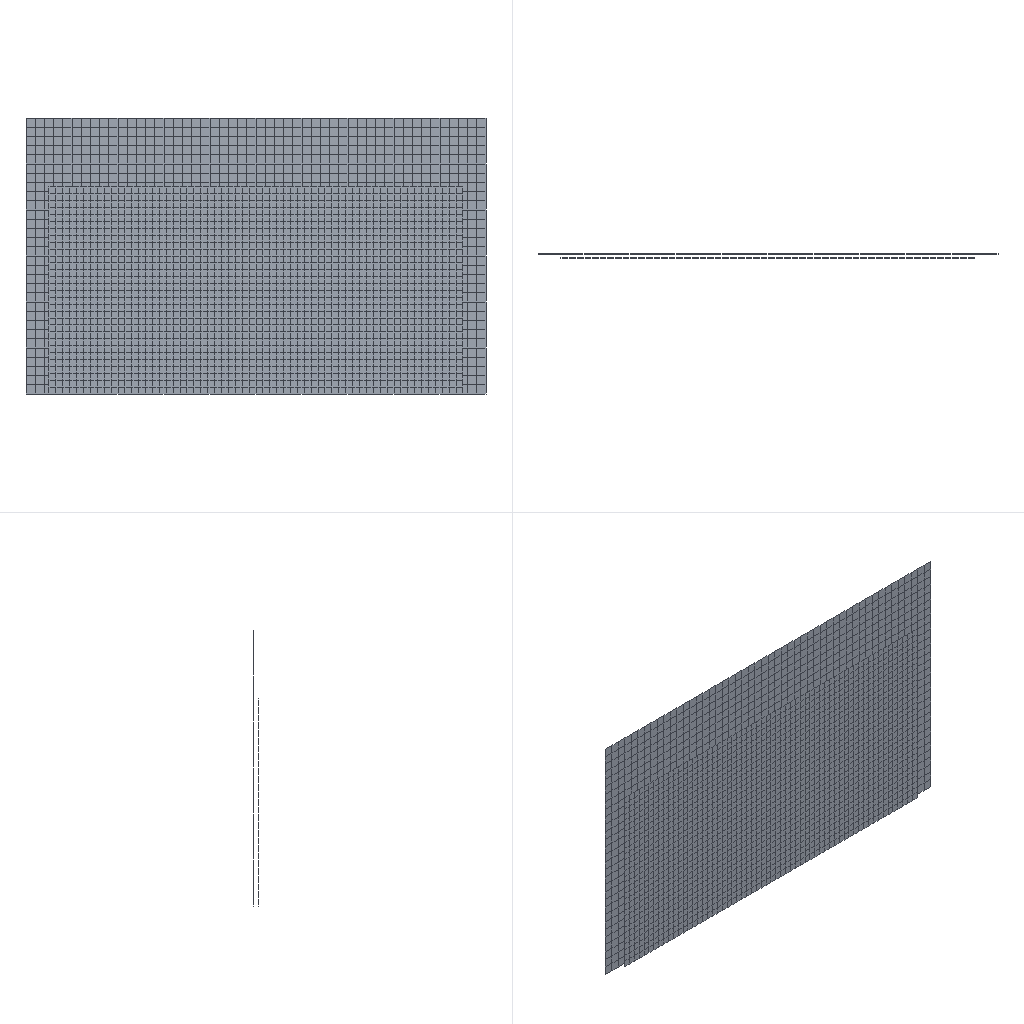Simulation study | abaqus
Set-up summary:
category,name,step,type,value,unit,region
solver,abaqus,,Abaqus/CAE 2024
units,mm-N-s-tonne (MPa),,inferred,E=70000 density=2.7e-09
analysis,forming step,,dynamic explicit,nlgeom=True; time_period=0.1
mesh,nodes,,,3941
mesh,elements,,,3720
element_type,S4R,,,3300
element_type,R3D4,,,420
material,banliao,,E,70000
material,banliao,,nu,0.33
material,banliao,,density,2.7e-09
material,banliao,,yield,131
material,banliao,,behaviors,plastic
material,xiangpi,,density,1.6e-09
material,xiangpi,,behaviors,hyperelastic
section,banliao,,shell section,2,,_PickedSet2
section,xiangpi,,shell section,10,,_PickedSet4
load,pressure,forming step,pressure,-5,,Surf-1
bc,fixdown,initial,encastre,[dofs=ENCASTRE],,down
contact,general,initial,general contact,interaction=Friction; friction=0.1; behavior=hard
constraint,rigid body,,,1
Abaqus input file, long lists of numbers shortened:
*Heading
** Job name: deck Model name: Model-1
** Generated by: Abaqus/CAE 2024
*Preprint, echo=NO, model=NO, history=NO, contact=NO
**
** PARTS
**
*Part, name=banliao
*Node
      1,         450.,         150.,         450.
      2,         435.,         150.,         450.
** (1889 more lines like these left out)
*Element, type=S4R
   1,    1,    2,   63,   62
   2,    2,    3,   64,   63
** (1798 more lines like these left out)
*Nset, nset=_PickedSet2, internal, generate
    1,  1891,     1
*Elset, elset=_PickedSet2, internal, generate
    1,  1800,     1
*Nset, nset=bl, generate
    1,  1891,     1
*Elset, elset=bl, generate
    1,  1800,     1
** Section: AIsection
*Shell Section, elset=_PickedSet2, material=banliao
2., 5
*End Part
**
*Part, name=muju
*Node
      1,        -240.,           0.,         500.
      2,        -250.,         -10.,         500.
** (466 more lines like these left out)
*Element, type=R3D4
 1,   1,  17, 161,  44
 2,  17,  18, 162, 161
** (418 more lines like these left out)
*Node
    469,         250.,        -150.,         250.
*Nset, nset=muju-RefPt_, internal
469,
*Nset, nset=down
 469,
*Elset, elset=muju, generate
   1,  420,    1
*End Part
**
*Part, name=xiangpi
*Node
      1,         500.,         250.,         600.
      2,         480.,         250.,         600.
** (1579 more lines like these left out)
*Element, type=S4R
   1,    1,    2,   53,   52
   2,    2,    3,   54,   53
** (1498 more lines like these left out)
*Nset, nset=xp, generate
    1,  1581,     1
*Elset, elset=xp, generate
    1,  1500,     1
*Nset, nset=_PickedSet3, internal, generate
    1,  1581,     1
*Elset, elset=_PickedSet3, internal, generate
    1,  1500,     1
*Nset, nset=_PickedSet4, internal, generate
    1,  1581,     1
*Elset, elset=_PickedSet4, internal, generate
    1,  1500,     1
** Section: Rub-section
*Shell Section, elset=_PickedSet4, material=xiangpi, controls=EC-1
10., 5
*End Part
**
**
** ASSEMBLY
**
*Assembly, name=Assembly
**
*Instance, name=banliao-1, part=banliao
          0.,        -148.,           0.
*End Instance
**
*Instance, name=muju-1, part=muju
*End Instance
**
*Instance, name=xiangpi-1, part=xiangpi
          0.,        -239.,           0.
*End Instance
**
*Nset, nset=down, instance=muju-1
 469,
*Elset, elset=_Surf-1_SPOS, internal, instance=xiangpi-1, generate
    1,  1500,     1
*Surface, type=ELEMENT, name=Surf-1
_Surf-1_SPOS, SPOS
*Rigid Body, ref node=muju-1.muju-RefPt_, elset=muju-1.muju
*End Assembly
**
** ELEMENT CONTROLS
**
*Section Controls, name=EC-1, hourglass=ENHANCED
1., 1., 1.
*Amplitude, name=Amp-1, definition=SMOOTH STEP
             0.,              0.,             0.1,              1.
**
** MATERIALS
**
*Material, name=banliao
*Density
 2.7e-09,
*Elastic
70000., 0.33
*Plastic
131.,0.
*Material, name=xiangpi
*Density
 1.6e-09,
*Hyperelastic, reduced polynomial
50.,0.
**
** INTERACTION PROPERTIES
**
*Surface Interaction, name=Friction
*Friction
 0.1,
*Surface Behavior, pressure-overclosure=HARD
**
** BOUNDARY CONDITIONS
**
** Name: fixdown Type: Symmetry/Antisymmetry/Encastre
*Boundary
down, ENCASTRE
**
** INTERACTIONS
**
** Interaction: general contact
*Contact, op=NEW
*Contact Inclusions, ALL EXTERIOR
*Contact Property Assignment
 ,  , Friction
** ----------------------------------------------------------------
**
** STEP: forming step
**
*Step, name="forming step", nlgeom=YES
*Dynamic, Explicit
, 0.1
*Bulk Viscosity
0.06, 1.2
** Mass Scaling: Semi-Automatic
**               Whole Model
*Fixed Mass Scaling, factor=1000.
**
** LOADS
**
** Name: pressure   Type: Pressure
*Dsload, amplitude=Amp-1
Surf-1, P, -5.
**
** OUTPUT REQUESTS
**
*Restart, write, number interval=1, time marks=NO
**
** FIELD OUTPUT: thickness
**
*Output, field
*Element Output, elset=banliao-1.bl, directions=YES
STH,
**
** FIELD OUTPUT: F-Output-1
**
*Output, field, variable=PRESELECT
**
** HISTORY OUTPUT: reactive force
**
*Output, history
*Node Output, nset=down
CF1, CF2, CF3, CM1, CM2, CM3, RF1, RF2
RF3, RM, RM1, RM2, RM3, RT, RWM
**
** HISTORY OUTPUT: H-Output-1
**
*Output, history, variable=PRESELECT
*End Step
Results summary:
result,odb.job_status,,,JOB_STATUS_COMPLETED_SUCCESSFULLY,"consistent, unstated (Abaqus has no unit system)"
result,steps[0].procedure,forming step,,"*DYNAMIC, EXPLICIT","consistent, unstated (Abaqus has no unit system)"
result,steps[0].time_period,forming step,,0.1,"consistent, unstated (Abaqus has no unit system)"
result,steps[0].n_frames,forming step,,21,"consistent, unstated (Abaqus has no unit system)"
result,steps[0].last_frame.id,forming step,,1361,"consistent, unstated (Abaqus has no unit system)"
result,steps[0].last_frame.value,forming step,,0.1,"consistent, unstated (Abaqus has no unit system)"
result,steps[0].last_frame.description,forming step,,Increment      1361: Step Time =   0.1,"consistent, unstated (Abaqus has no unit system)"
result,steps[0].completed,forming step,,True,"consistent, unstated (Abaqus has no unit system)"
result,steps[0].max_U_magnitude,forming step,,339.748,"consistent, unstated (Abaqus has no unit system)"
result,steps[0].max_S_mises,forming step,,732.612,"consistent, unstated (Abaqus has no unit system)"
result,steps[0].RF_sum[1],forming step,,-7003.86,"consistent, unstated (Abaqus has no unit system)"
result,steps[0].RF_sum[2],forming step,,1.45222e+06,"consistent, unstated (Abaqus has no unit system)"
result,steps[0].RF_sum[3],forming step,,867978,"consistent, unstated (Abaqus has no unit system)"
result,steps[0].diagnostic.n_increments,forming step,,21,"consistent, unstated (Abaqus has no unit system)"